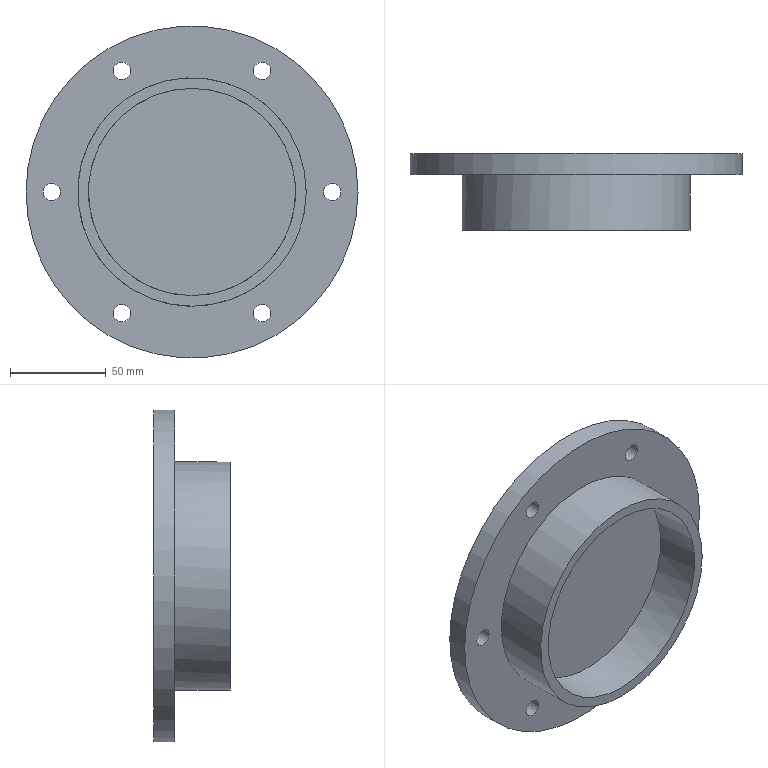Part | NX | features DATUM_CSYS 9, HOLE PACKAGE 9, SIMPLE HOLE 9, SKETCH 8, EXTRACT_DATUM_AXIS 6, EXTRACT_FACE 6, Instance Feature 5, EXTRUDE 2, DELETE FACE 1, OFFSET_REGION 1, Pattern Feature 1 | 1 solid | 15 faces | box 173 x 40 x 173 mm | volume 317265 mm3 | cylinder 10 | plane 5 | commonest cylinder face diameters 9 x6 108 x1 114 x1 119 x1 173 x1
STEP:
#1=CARTESIAN_POINT('',(86.5,-11.,0.));
#2=VERTEX_POINT('',#1);
#3=CARTESIAN_POINT('',(0.,-11.,0.));
#4=DIRECTION('',(0.,-1.,0.));
#5=DIRECTION('',(1.,0.,0.));
#6=AXIS2_PLACEMENT_3D('',#3,#4,#5);
#7=CIRCLE('',#6,86.5);
#8=EDGE_CURVE('',#2,#2,#7,.T.);
#9=ORIENTED_EDGE('',*,*,#8,.F.);
#10=EDGE_LOOP('',(#9));
#11=FACE_BOUND('',#10,.T.);
#12=CARTESIAN_POINT('',(86.5,0.,0.));
#13=VERTEX_POINT('',#12);
#14=CARTESIAN_POINT('',(0.,0.,0.));
#15=DIRECTION('',(0.,-1.,0.));
#16=DIRECTION('',(1.,0.,0.));
#17=AXIS2_PLACEMENT_3D('',#14,#15,#16);
#18=CIRCLE('',#17,86.5);
#19=EDGE_CURVE('',#13,#13,#18,.T.);
#20=ORIENTED_EDGE('',*,*,#19,.T.);
#21=EDGE_LOOP('',(#20));
#22=FACE_BOUND('',#21,.T.);
#23=CARTESIAN_POINT('',(0.,-11.,0.));
#24=DIRECTION('',(0.,1.,0.));
#25=DIRECTION('',(0.,0.,1.));
#26=AXIS2_PLACEMENT_3D('',#23,#24,#25);
#27=CYLINDRICAL_SURFACE('',#26,86.5);
#28=ADVANCED_FACE('',(#11,#22),#27,.T.);
#29=CARTESIAN_POINT('',(-36.5,-11.,-67.72));
#30=VERTEX_POINT('',#29);
#31=CARTESIAN_POINT('',(-36.5,-11.,-63.22));
#32=DIRECTION('',(0.,-1.,0.));
#33=DIRECTION('',(0.,0.,-1.));
#34=AXIS2_PLACEMENT_3D('',#31,#32,#33);
#35=CIRCLE('',#34,4.5);
#36=EDGE_CURVE('',#30,#30,#35,.T.);
#37=ORIENTED_EDGE('',*,*,#36,.F.);
#38=EDGE_LOOP('',(#37));
#39=FACE_BOUND('',#38,.T.);
#40=CARTESIAN_POINT('',(36.5,-11.,-67.72));
#41=VERTEX_POINT('',#40);
#42=CARTESIAN_POINT('',(36.5,-11.,-63.22));
#43=DIRECTION('',(0.,-1.,0.));
#44=DIRECTION('',(0.,0.,-1.));
#45=AXIS2_PLACEMENT_3D('',#42,#43,#44);
#46=CIRCLE('',#45,4.5);
#47=EDGE_CURVE('',#41,#41,#46,.T.);
#48=ORIENTED_EDGE('',*,*,#47,.F.);
#49=EDGE_LOOP('',(#48));
#50=FACE_BOUND('',#49,.T.);
#51=CARTESIAN_POINT('',(73.,-11.,-4.5));
#52=VERTEX_POINT('',#51);
#53=CARTESIAN_POINT('',(73.,-11.,0.));
#54=DIRECTION('',(0.,-1.,0.));
#55=DIRECTION('',(0.,0.,-1.));
#56=AXIS2_PLACEMENT_3D('',#53,#54,#55);
#57=CIRCLE('',#56,4.5);
#58=EDGE_CURVE('',#52,#52,#57,.T.);
#59=ORIENTED_EDGE('',*,*,#58,.F.);
#60=EDGE_LOOP('',(#59));
#61=FACE_BOUND('',#60,.T.);
#62=CARTESIAN_POINT('',(36.5,-11.,58.72));
#63=VERTEX_POINT('',#62);
#64=CARTESIAN_POINT('',(36.5,-11.,63.22));
#65=DIRECTION('',(0.,-1.,0.));
#66=DIRECTION('',(0.,0.,-1.));
#67=AXIS2_PLACEMENT_3D('',#64,#65,#66);
#68=CIRCLE('',#67,4.5);
#69=EDGE_CURVE('',#63,#63,#68,.T.);
#70=ORIENTED_EDGE('',*,*,#69,.F.);
#71=EDGE_LOOP('',(#70));
#72=FACE_BOUND('',#71,.T.);
#73=CARTESIAN_POINT('',(-36.5,-11.,58.72));
#74=VERTEX_POINT('',#73);
#75=CARTESIAN_POINT('',(-36.5,-11.,63.22));
#76=DIRECTION('',(0.,-1.,0.));
#77=DIRECTION('',(0.,0.,-1.));
#78=AXIS2_PLACEMENT_3D('',#75,#76,#77);
#79=CIRCLE('',#78,4.5);
#80=EDGE_CURVE('',#74,#74,#79,.T.);
#81=ORIENTED_EDGE('',*,*,#80,.F.);
#82=EDGE_LOOP('',(#81));
#83=FACE_BOUND('',#82,.T.);
#84=CARTESIAN_POINT('',(-73.,-11.,-4.5));
#85=VERTEX_POINT('',#84);
#86=CARTESIAN_POINT('',(-73.,-11.,0.));
#87=DIRECTION('',(0.,-1.,0.));
#88=DIRECTION('',(0.,0.,-1.));
#89=AXIS2_PLACEMENT_3D('',#86,#87,#88);
#90=CIRCLE('',#89,4.5);
#91=EDGE_CURVE('',#85,#85,#90,.T.);
#92=ORIENTED_EDGE('',*,*,#91,.F.);
#93=EDGE_LOOP('',(#92));
#94=FACE_BOUND('',#93,.T.);
#95=CARTESIAN_POINT('',(59.5,-11.,0.));
#96=VERTEX_POINT('',#95);
#97=CARTESIAN_POINT('',(0.,-11.,0.));
#98=DIRECTION('',(0.,-1.,0.));
#99=DIRECTION('',(1.,0.,0.));
#100=AXIS2_PLACEMENT_3D('',#97,#98,#99);
#101=CIRCLE('',#100,59.5);
#102=EDGE_CURVE('',#96,#96,#101,.T.);
#103=ORIENTED_EDGE('',*,*,#102,.F.);
#104=EDGE_LOOP('',(#103));
#105=FACE_BOUND('',#104,.T.);
#106=ORIENTED_EDGE('',*,*,#8,.T.);
#107=EDGE_LOOP('',(#106));
#108=FACE_BOUND('',#107,.T.);
#109=CARTESIAN_POINT('',(0.,-11.,0.));
#110=DIRECTION('',(0.,-1.,0.));
#111=DIRECTION('',(0.,0.,-1.));
#112=AXIS2_PLACEMENT_3D('',#109,#110,#111);
#113=PLANE('',#112);
#114=ADVANCED_FACE('',(#39,#50,#61,#72,#83,#94,#105,#108),#113,.T.);
#115=CARTESIAN_POINT('',(-36.5,0.,-67.72));
#116=VERTEX_POINT('',#115);
#117=CARTESIAN_POINT('',(-36.5,0.,-63.22));
#118=DIRECTION('',(0.,-1.,0.));
#119=DIRECTION('',(0.,0.,-1.));
#120=AXIS2_PLACEMENT_3D('',#117,#118,#119);
#121=CIRCLE('',#120,4.5);
#122=EDGE_CURVE('',#116,#116,#121,.T.);
#123=ORIENTED_EDGE('',*,*,#122,.T.);
#124=EDGE_LOOP('',(#123));
#125=FACE_BOUND('',#124,.T.);
#126=CARTESIAN_POINT('',(36.5,0.,-67.72));
#127=VERTEX_POINT('',#126);
#128=CARTESIAN_POINT('',(36.5,0.,-63.22));
#129=DIRECTION('',(0.,-1.,0.));
#130=DIRECTION('',(0.,0.,-1.));
#131=AXIS2_PLACEMENT_3D('',#128,#129,#130);
#132=CIRCLE('',#131,4.5);
#133=EDGE_CURVE('',#127,#127,#132,.T.);
#134=ORIENTED_EDGE('',*,*,#133,.T.);
#135=EDGE_LOOP('',(#134));
#136=FACE_BOUND('',#135,.T.);
#137=CARTESIAN_POINT('',(73.,0.,-4.5));
#138=VERTEX_POINT('',#137);
#139=CARTESIAN_POINT('',(73.,0.,0.));
#140=DIRECTION('',(0.,-1.,0.));
#141=DIRECTION('',(0.,0.,-1.));
#142=AXIS2_PLACEMENT_3D('',#139,#140,#141);
#143=CIRCLE('',#142,4.5);
#144=EDGE_CURVE('',#138,#138,#143,.T.);
#145=ORIENTED_EDGE('',*,*,#144,.T.);
#146=EDGE_LOOP('',(#145));
#147=FACE_BOUND('',#146,.T.);
#148=CARTESIAN_POINT('',(36.5,0.,58.72));
#149=VERTEX_POINT('',#148);
#150=CARTESIAN_POINT('',(36.5,0.,63.22));
#151=DIRECTION('',(0.,-1.,0.));
#152=DIRECTION('',(0.,0.,-1.));
#153=AXIS2_PLACEMENT_3D('',#150,#151,#152);
#154=CIRCLE('',#153,4.5);
#155=EDGE_CURVE('',#149,#149,#154,.T.);
#156=ORIENTED_EDGE('',*,*,#155,.T.);
#157=EDGE_LOOP('',(#156));
#158=FACE_BOUND('',#157,.T.);
#159=CARTESIAN_POINT('',(-36.5,0.,58.72));
#160=VERTEX_POINT('',#159);
#161=CARTESIAN_POINT('',(-36.5,0.,63.22));
#162=DIRECTION('',(0.,-1.,0.));
#163=DIRECTION('',(0.,0.,-1.));
#164=AXIS2_PLACEMENT_3D('',#161,#162,#163);
#165=CIRCLE('',#164,4.5);
#166=EDGE_CURVE('',#160,#160,#165,.T.);
#167=ORIENTED_EDGE('',*,*,#166,.T.);
#168=EDGE_LOOP('',(#167));
#169=FACE_BOUND('',#168,.T.);
#170=CARTESIAN_POINT('',(-73.,0.,-4.5));
#171=VERTEX_POINT('',#170);
#172=CARTESIAN_POINT('',(-73.,0.,0.));
#173=DIRECTION('',(0.,-1.,0.));
#174=DIRECTION('',(0.,0.,-1.));
#175=AXIS2_PLACEMENT_3D('',#172,#173,#174);
#176=CIRCLE('',#175,4.5);
#177=EDGE_CURVE('',#171,#171,#176,.T.);
#178=ORIENTED_EDGE('',*,*,#177,.T.);
#179=EDGE_LOOP('',(#178));
#180=FACE_BOUND('',#179,.T.);
#181=CARTESIAN_POINT('',(0.,0.,-57.));
#182=VERTEX_POINT('',#181);
#183=CARTESIAN_POINT('',(0.,0.,0.));
#184=DIRECTION('',(0.,-1.,0.));
#185=DIRECTION('',(0.,0.,-1.));
#186=AXIS2_PLACEMENT_3D('',#183,#184,#185);
#187=CIRCLE('',#186,57.);
#188=EDGE_CURVE('',#182,#182,#187,.T.);
#189=ORIENTED_EDGE('',*,*,#188,.T.);
#190=EDGE_LOOP('',(#189));
#191=FACE_BOUND('',#190,.T.);
#192=ORIENTED_EDGE('',*,*,#19,.F.);
#193=EDGE_LOOP('',(#192));
#194=FACE_BOUND('',#193,.T.);
#195=CARTESIAN_POINT('',(0.,0.,0.));
#196=DIRECTION('',(0.,-1.,0.));
#197=DIRECTION('',(0.,0.,-1.));
#198=AXIS2_PLACEMENT_3D('',#195,#196,#197);
#199=PLANE('',#198);
#200=ADVANCED_FACE('',(#125,#136,#147,#158,#169,#180,#191,#194),#199,.F.);
#201=CARTESIAN_POINT('',(0.,-40.,-59.5));
#202=VERTEX_POINT('',#201);
#203=CARTESIAN_POINT('',(0.,-40.,0.));
#204=DIRECTION('',(0.,-1.,0.));
#205=DIRECTION('',(0.,0.,-1.));
#206=AXIS2_PLACEMENT_3D('',#203,#204,#205);
#207=CIRCLE('',#206,59.5);
#208=EDGE_CURVE('',#202,#202,#207,.T.);
#209=ORIENTED_EDGE('',*,*,#208,.F.);
#210=EDGE_LOOP('',(#209));
#211=FACE_BOUND('',#210,.T.);
#212=ORIENTED_EDGE('',*,*,#102,.T.);
#213=EDGE_LOOP('',(#212));
#214=FACE_BOUND('',#213,.T.);
#215=CARTESIAN_POINT('',(0.,-35.,0.));
#216=DIRECTION('',(0.,1.,0.));
#217=DIRECTION('',(0.,0.,1.));
#218=AXIS2_PLACEMENT_3D('',#215,#216,#217);
#219=CYLINDRICAL_SURFACE('',#218,59.5);
#220=ADVANCED_FACE('',(#211,#214),#219,.T.);
#221=CARTESIAN_POINT('',(0.,-40.,-54.));
#222=VERTEX_POINT('',#221);
#223=CARTESIAN_POINT('',(0.,-40.,0.));
#224=DIRECTION('',(0.,-1.,0.));
#225=DIRECTION('',(0.,0.,-1.));
#226=AXIS2_PLACEMENT_3D('',#223,#224,#225);
#227=CIRCLE('',#226,54.);
#228=EDGE_CURVE('',#222,#222,#227,.F.);
#229=ORIENTED_EDGE('',*,*,#228,.T.);
#230=EDGE_LOOP('',(#229));
#231=FACE_BOUND('',#230,.T.);
#232=ORIENTED_EDGE('',*,*,#208,.T.);
#233=EDGE_LOOP('',(#232));
#234=FACE_BOUND('',#233,.T.);
#235=CARTESIAN_POINT('',(0.,-40.,0.));
#236=DIRECTION('',(0.,-1.,0.));
#237=DIRECTION('',(0.,0.,-1.));
#238=AXIS2_PLACEMENT_3D('',#235,#236,#237);
#239=PLANE('',#238);
#240=ADVANCED_FACE('',(#231,#234),#239,.T.);
#241=CARTESIAN_POINT('',(0.,-15.,54.));
#242=VERTEX_POINT('',#241);
#243=CARTESIAN_POINT('',(0.,-15.,0.));
#244=DIRECTION('',(0.,1.,0.));
#245=DIRECTION('',(0.,0.,1.));
#246=AXIS2_PLACEMENT_3D('',#243,#244,#245);
#247=CIRCLE('',#246,54.);
#248=EDGE_CURVE('',#242,#242,#247,.F.);
#249=ORIENTED_EDGE('',*,*,#248,.T.);
#250=EDGE_LOOP('',(#249));
#251=FACE_BOUND('',#250,.T.);
#252=CARTESIAN_POINT('',(0.,-15.,0.));
#253=DIRECTION('',(0.,1.,0.));
#254=DIRECTION('',(0.,0.,1.));
#255=AXIS2_PLACEMENT_3D('',#252,#253,#254);
#256=PLANE('',#255);
#257=ADVANCED_FACE('',(#251),#256,.F.);
#258=ORIENTED_EDGE('',*,*,#248,.F.);
#259=EDGE_LOOP('',(#258));
#260=FACE_BOUND('',#259,.T.);
#261=ORIENTED_EDGE('',*,*,#228,.F.);
#262=EDGE_LOOP('',(#261));
#263=FACE_BOUND('',#262,.T.);
#264=CARTESIAN_POINT('',(0.,-35.,0.));
#265=DIRECTION('',(0.,1.,0.));
#266=DIRECTION('',(0.,0.,1.));
#267=AXIS2_PLACEMENT_3D('',#264,#265,#266);
#268=CYLINDRICAL_SURFACE('',#267,54.);
#269=ADVANCED_FACE('',(#260,#263),#268,.F.);
#270=CARTESIAN_POINT('',(0.,-3.,-57.));
#271=VERTEX_POINT('',#270);
#272=CARTESIAN_POINT('',(0.,-3.,0.));
#273=DIRECTION('',(0.,-1.,0.));
#274=DIRECTION('',(0.,0.,-1.));
#275=AXIS2_PLACEMENT_3D('',#272,#273,#274);
#276=CIRCLE('',#275,57.);
#277=EDGE_CURVE('',#271,#271,#276,.F.);
#278=ORIENTED_EDGE('',*,*,#277,.T.);
#279=EDGE_LOOP('',(#278));
#280=FACE_BOUND('',#279,.T.);
#281=CARTESIAN_POINT('',(0.,-3.,0.));
#282=DIRECTION('',(0.,-1.,0.));
#283=DIRECTION('',(0.,0.,-1.));
#284=AXIS2_PLACEMENT_3D('',#281,#282,#283);
#285=PLANE('',#284);
#286=ADVANCED_FACE('',(#280),#285,.F.);
#287=ORIENTED_EDGE('',*,*,#277,.F.);
#288=EDGE_LOOP('',(#287));
#289=FACE_BOUND('',#288,.T.);
#290=ORIENTED_EDGE('',*,*,#188,.F.);
#291=EDGE_LOOP('',(#290));
#292=FACE_BOUND('',#291,.T.);
#293=CARTESIAN_POINT('',(0.,0.,0.));
#294=DIRECTION('',(0.,-1.,0.));
#295=DIRECTION('',(0.,0.,-1.));
#296=AXIS2_PLACEMENT_3D('',#293,#294,#295);
#297=CYLINDRICAL_SURFACE('',#296,57.);
#298=ADVANCED_FACE('',(#289,#292),#297,.F.);
#299=ORIENTED_EDGE('',*,*,#91,.T.);
#300=EDGE_LOOP('',(#299));
#301=FACE_BOUND('',#300,.T.);
#302=ORIENTED_EDGE('',*,*,#177,.F.);
#303=EDGE_LOOP('',(#302));
#304=FACE_BOUND('',#303,.T.);
#305=CARTESIAN_POINT('',(-73.,0.,0.));
#306=DIRECTION('',(0.,-1.,0.));
#307=DIRECTION('',(0.,0.,-1.));
#308=AXIS2_PLACEMENT_3D('',#305,#306,#307);
#309=CYLINDRICAL_SURFACE('',#308,4.5);
#310=ADVANCED_FACE('',(#301,#304),#309,.F.);
#311=ORIENTED_EDGE('',*,*,#80,.T.);
#312=EDGE_LOOP('',(#311));
#313=FACE_BOUND('',#312,.T.);
#314=ORIENTED_EDGE('',*,*,#166,.F.);
#315=EDGE_LOOP('',(#314));
#316=FACE_BOUND('',#315,.T.);
#317=CARTESIAN_POINT('',(-36.5,0.,63.22));
#318=DIRECTION('',(0.,-1.,0.));
#319=DIRECTION('',(0.,0.,-1.));
#320=AXIS2_PLACEMENT_3D('',#317,#318,#319);
#321=CYLINDRICAL_SURFACE('',#320,4.5);
#322=ADVANCED_FACE('',(#313,#316),#321,.F.);
#323=ORIENTED_EDGE('',*,*,#69,.T.);
#324=EDGE_LOOP('',(#323));
#325=FACE_BOUND('',#324,.T.);
#326=ORIENTED_EDGE('',*,*,#155,.F.);
#327=EDGE_LOOP('',(#326));
#328=FACE_BOUND('',#327,.T.);
#329=CARTESIAN_POINT('',(36.5,0.,63.22));
#330=DIRECTION('',(0.,-1.,0.));
#331=DIRECTION('',(0.,0.,-1.));
#332=AXIS2_PLACEMENT_3D('',#329,#330,#331);
#333=CYLINDRICAL_SURFACE('',#332,4.5);
#334=ADVANCED_FACE('',(#325,#328),#333,.F.);
#335=ORIENTED_EDGE('',*,*,#58,.T.);
#336=EDGE_LOOP('',(#335));
#337=FACE_BOUND('',#336,.T.);
#338=ORIENTED_EDGE('',*,*,#144,.F.);
#339=EDGE_LOOP('',(#338));
#340=FACE_BOUND('',#339,.T.);
#341=CARTESIAN_POINT('',(73.,0.,0.));
#342=DIRECTION('',(0.,-1.,0.));
#343=DIRECTION('',(0.,0.,-1.));
#344=AXIS2_PLACEMENT_3D('',#341,#342,#343);
#345=CYLINDRICAL_SURFACE('',#344,4.5);
#346=ADVANCED_FACE('',(#337,#340),#345,.F.);
#347=ORIENTED_EDGE('',*,*,#47,.T.);
#348=EDGE_LOOP('',(#347));
#349=FACE_BOUND('',#348,.T.);
#350=ORIENTED_EDGE('',*,*,#133,.F.);
#351=EDGE_LOOP('',(#350));
#352=FACE_BOUND('',#351,.T.);
#353=CARTESIAN_POINT('',(36.5,0.,-63.22));
#354=DIRECTION('',(0.,-1.,0.));
#355=DIRECTION('',(0.,0.,-1.));
#356=AXIS2_PLACEMENT_3D('',#353,#354,#355);
#357=CYLINDRICAL_SURFACE('',#356,4.5);
#358=ADVANCED_FACE('',(#349,#352),#357,.F.);
#359=ORIENTED_EDGE('',*,*,#36,.T.);
#360=EDGE_LOOP('',(#359));
#361=FACE_BOUND('',#360,.T.);
#362=ORIENTED_EDGE('',*,*,#122,.F.);
#363=EDGE_LOOP('',(#362));
#364=FACE_BOUND('',#363,.T.);
#365=CARTESIAN_POINT('',(-36.5,0.,-63.22));
#366=DIRECTION('',(0.,-1.,0.));
#367=DIRECTION('',(0.,0.,-1.));
#368=AXIS2_PLACEMENT_3D('',#365,#366,#367);
#369=CYLINDRICAL_SURFACE('',#368,4.5);
#370=ADVANCED_FACE('',(#361,#364),#369,.F.);
#371=CLOSED_SHELL('',(#28,#114,#200,#220,#240,#257,#269,#286,#298,#310,#322,#334,#346,#358,#370));
#372=MANIFOLD_SOLID_BREP('',#371);
#373=(LENGTH_UNIT()NAMED_UNIT(*)SI_UNIT(.MILLI.,.METRE.));
#374=UNCERTAINTY_MEASURE_WITH_UNIT(LENGTH_MEASURE(0.00001),#373,'','');
#375=(NAMED_UNIT(*)PLANE_ANGLE_UNIT()SI_UNIT($,.RADIAN.));
#376=(NAMED_UNIT(*)SI_UNIT($,.STERADIAN.)SOLID_ANGLE_UNIT());
#377=(GEOMETRIC_REPRESENTATION_CONTEXT(3)GLOBAL_UNCERTAINTY_ASSIGNED_CONTEXT((#374))GLOBAL_UNIT_ASSIGNED_CONTEXT((#373,#375,#376))REPRESENTATION_CONTEXT('',''));
#378=ADVANCED_BREP_SHAPE_REPRESENTATION('',(#372),#377);